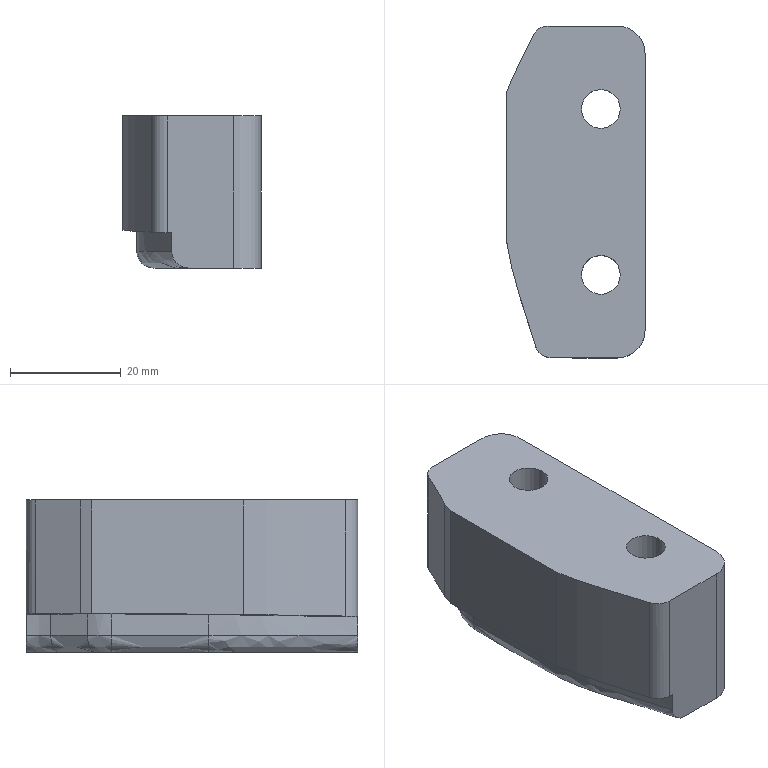Part | STEP file | gslz 2016.10.28-10_id2330_x_t | 1 solid | 30 faces | box 25 x 60 x 27.5 mm | volume 33698 mm3 | spline 14 | cylinder 8 | plane 8 | commonest cylinder face diameters 6 x2 7 x2 10 x2 11 x2